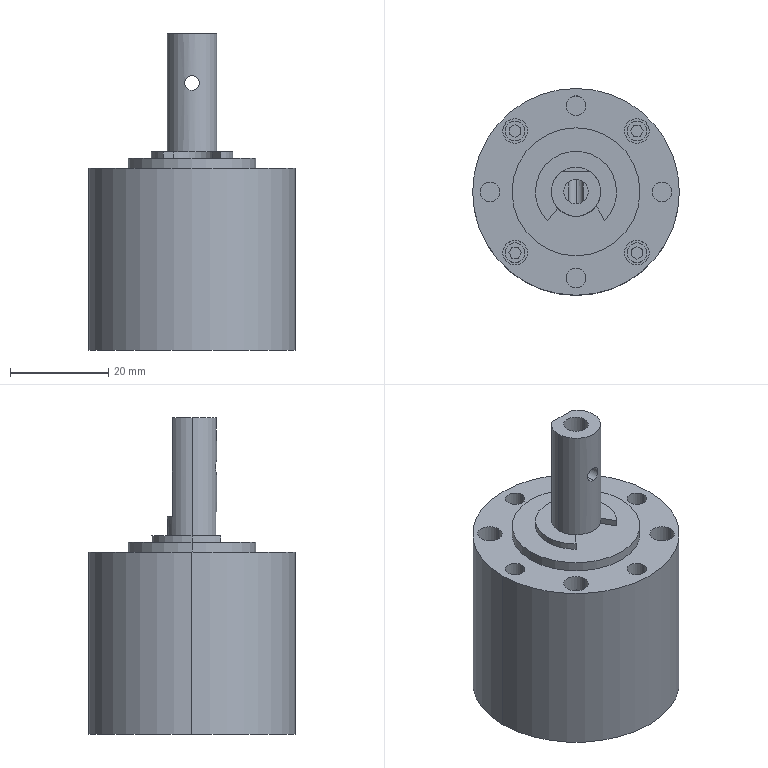Part | SolidWorks | features BaseBody 2 | 2 solids | 92 faces | box 42 x 42 x 64.3 mm | volume 52956 mm3 | plane 52 | cylinder 40 | commonest cylinder face diameters 4 x16 5 x10 10 x5 16.5 x3 3 x2 26 x2